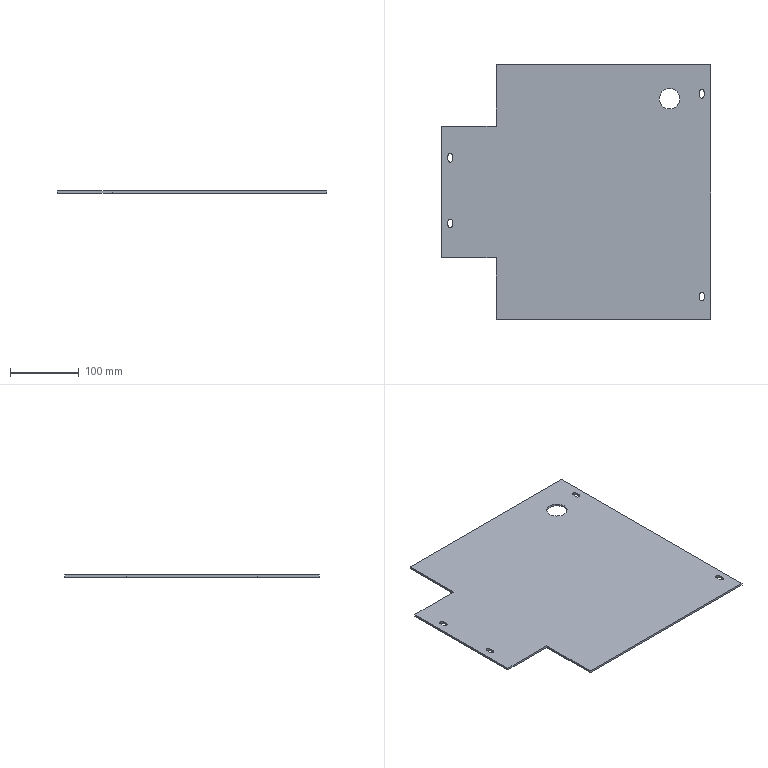Part | SolidWorks | features Cut 2, ICE 2, Extrusion 1 | 1 solid | 28 faces | box 393 x 372 x 3 mm | volume 392382 mm3 | plane 18 | cylinder 10 | commonest cylinder face diameters 6.6 x8 30 x2
STEP:
#1=CARTESIAN_POINT('',(106.5,136.,0.));
#2=VERTEX_POINT('',#1);
#3=CARTESIAN_POINT('',(136.5,136.,0.));
#4=VERTEX_POINT('',#3);
#5=CARTESIAN_POINT('',(121.5,136.,0.));
#6=DIRECTION('',(0.,0.,1.));
#7=DIRECTION('',(1.,0.,0.));
#8=AXIS2_PLACEMENT_3D('',#5,#6,#7);
#9=CIRCLE('',#8,15.);
#10=EDGE_CURVE('',#2,#4,#9,.T.);
#11=ORIENTED_EDGE('',*,*,#10,.F.);
#12=CARTESIAN_POINT('',(106.5,136.,3.));
#13=VERTEX_POINT('',#12);
#14=CARTESIAN_POINT('',(106.5,136.,-7.));
#15=DIRECTION('',(0.,0.,1.));
#16=VECTOR('',#15,1000.);
#17=LINE('',#14,#16);
#18=EDGE_CURVE('',#2,#13,#17,.T.);
#19=ORIENTED_EDGE('',*,*,#18,.T.);
#20=CARTESIAN_POINT('',(136.5,136.,3.));
#21=VERTEX_POINT('',#20);
#22=CARTESIAN_POINT('',(121.5,136.,3.));
#23=DIRECTION('',(0.,0.,1.));
#24=DIRECTION('',(1.,0.,0.));
#25=AXIS2_PLACEMENT_3D('',#22,#23,#24);
#26=CIRCLE('',#25,15.);
#27=EDGE_CURVE('',#13,#21,#26,.T.);
#28=ORIENTED_EDGE('',*,*,#27,.T.);
#29=CARTESIAN_POINT('',(136.5,136.,-7.));
#30=DIRECTION('',(0.,0.,1.));
#31=VECTOR('',#30,1000.);
#32=LINE('',#29,#31);
#33=EDGE_CURVE('',#4,#21,#32,.T.);
#34=ORIENTED_EDGE('',*,*,#33,.F.);
#35=EDGE_LOOP('',(#11,#19,#28,#34));
#36=FACE_OUTER_BOUND('',#35,.T.);
#37=CARTESIAN_POINT('',(121.5,136.,-7.));
#38=DIRECTION('',(0.,0.,1.));
#39=DIRECTION('',(1.,0.,0.));
#40=AXIS2_PLACEMENT_3D('',#37,#38,#39);
#41=CYLINDRICAL_SURFACE('',#40,15.);
#42=ADVANCED_FACE('',(#36),#41,.F.);
#43=CARTESIAN_POINT('',(-131.5,-186.,3.));
#44=VERTEX_POINT('',#43);
#45=CARTESIAN_POINT('',(181.5,-186.,3.));
#46=VERTEX_POINT('',#45);
#47=CARTESIAN_POINT('',(181.5,-186.,3.));
#48=DIRECTION('',(1.,0.,0.));
#49=VECTOR('',#48,1000.);
#50=LINE('',#47,#49);
#51=EDGE_CURVE('',#44,#46,#50,.T.);
#52=ORIENTED_EDGE('',*,*,#51,.F.);
#53=CARTESIAN_POINT('',(-131.5,-186.,0.));
#54=VERTEX_POINT('',#53);
#55=CARTESIAN_POINT('',(-131.5,-186.,-7.));
#56=DIRECTION('',(0.,0.,1.));
#57=VECTOR('',#56,1000.);
#58=LINE('',#55,#57);
#59=EDGE_CURVE('',#54,#44,#58,.T.);
#60=ORIENTED_EDGE('',*,*,#59,.F.);
#61=CARTESIAN_POINT('',(181.5,-186.,0.));
#62=VERTEX_POINT('',#61);
#63=CARTESIAN_POINT('',(181.5,-186.,0.));
#64=DIRECTION('',(1.,0.,0.));
#65=VECTOR('',#64,1000.);
#66=LINE('',#63,#65);
#67=EDGE_CURVE('',#54,#62,#66,.T.);
#68=ORIENTED_EDGE('',*,*,#67,.T.);
#69=CARTESIAN_POINT('',(181.5,-186.,3.));
#70=DIRECTION('',(0.,0.,-1.));
#71=VECTOR('',#70,1000.);
#72=LINE('',#69,#71);
#73=EDGE_CURVE('',#46,#62,#72,.T.);
#74=ORIENTED_EDGE('',*,*,#73,.F.);
#75=EDGE_LOOP('',(#52,#60,#68,#74));
#76=FACE_OUTER_BOUND('',#75,.T.);
#77=CARTESIAN_POINT('',(181.5,-186.,3.));
#78=DIRECTION('',(0.,1.,0.));
#79=DIRECTION('',(-1.,0.,0.));
#80=AXIS2_PLACEMENT_3D('',#77,#78,#79);
#81=PLANE('',#80);
#82=ADVANCED_FACE('',(#76),#81,.F.);
#83=CARTESIAN_POINT('',(181.5,186.,0.));
#84=VERTEX_POINT('',#83);
#85=CARTESIAN_POINT('',(181.5,-186.,0.));
#86=DIRECTION('',(0.,1.,0.));
#87=VECTOR('',#86,1000.);
#88=LINE('',#85,#87);
#89=EDGE_CURVE('',#62,#84,#88,.T.);
#90=ORIENTED_EDGE('',*,*,#89,.T.);
#91=CARTESIAN_POINT('',(181.5,186.,3.));
#92=VERTEX_POINT('',#91);
#93=CARTESIAN_POINT('',(181.5,186.,3.));
#94=DIRECTION('',(0.,0.,-1.));
#95=VECTOR('',#94,1000.);
#96=LINE('',#93,#95);
#97=EDGE_CURVE('',#92,#84,#96,.T.);
#98=ORIENTED_EDGE('',*,*,#97,.F.);
#99=CARTESIAN_POINT('',(181.5,-186.,3.));
#100=DIRECTION('',(0.,1.,0.));
#101=VECTOR('',#100,1000.);
#102=LINE('',#99,#101);
#103=EDGE_CURVE('',#46,#92,#102,.T.);
#104=ORIENTED_EDGE('',*,*,#103,.F.);
#105=ORIENTED_EDGE('',*,*,#73,.T.);
#106=EDGE_LOOP('',(#90,#98,#104,#105));
#107=FACE_OUTER_BOUND('',#106,.T.);
#108=CARTESIAN_POINT('',(181.5,-186.,3.));
#109=DIRECTION('',(-1.,0.,0.));
#110=DIRECTION('',(0.,0.,1.));
#111=AXIS2_PLACEMENT_3D('',#108,#109,#110);
#112=PLANE('',#111);
#113=ADVANCED_FACE('',(#107),#112,.F.);
#114=CARTESIAN_POINT('',(-131.5,186.,0.));
#115=VERTEX_POINT('',#114);
#116=CARTESIAN_POINT('',(181.5,186.,0.));
#117=DIRECTION('',(-1.,0.,0.));
#118=VECTOR('',#117,1000.);
#119=LINE('',#116,#118);
#120=EDGE_CURVE('',#84,#115,#119,.T.);
#121=ORIENTED_EDGE('',*,*,#120,.T.);
#122=CARTESIAN_POINT('',(-131.5,186.,3.));
#123=VERTEX_POINT('',#122);
#124=CARTESIAN_POINT('',(-131.5,186.,-7.));
#125=DIRECTION('',(0.,0.,1.));
#126=VECTOR('',#125,1000.);
#127=LINE('',#124,#126);
#128=EDGE_CURVE('',#115,#123,#127,.T.);
#129=ORIENTED_EDGE('',*,*,#128,.T.);
#130=CARTESIAN_POINT('',(181.5,186.,3.));
#131=DIRECTION('',(-1.,0.,0.));
#132=VECTOR('',#131,1000.);
#133=LINE('',#130,#132);
#134=EDGE_CURVE('',#92,#123,#133,.T.);
#135=ORIENTED_EDGE('',*,*,#134,.F.);
#136=ORIENTED_EDGE('',*,*,#97,.T.);
#137=EDGE_LOOP('',(#121,#129,#135,#136));
#138=FACE_OUTER_BOUND('',#137,.T.);
#139=CARTESIAN_POINT('',(181.5,186.,3.));
#140=DIRECTION('',(0.,-1.,0.));
#141=DIRECTION('',(1.,0.,0.));
#142=AXIS2_PLACEMENT_3D('',#139,#140,#141);
#143=PLANE('',#142);
#144=ADVANCED_FACE('',(#138),#143,.F.);
#145=CARTESIAN_POINT('',(165.2,-155.558,3.));
#146=VERTEX_POINT('',#145);
#147=CARTESIAN_POINT('',(171.8,-155.558,3.));
#148=VERTEX_POINT('',#147);
#149=CARTESIAN_POINT('',(168.5,-155.558,3.));
#150=DIRECTION('',(0.,0.,1.));
#151=DIRECTION('',(1.,0.,0.));
#152=AXIS2_PLACEMENT_3D('',#149,#150,#151);
#153=CIRCLE('',#152,3.3);
#154=EDGE_CURVE('',#146,#148,#153,.T.);
#155=ORIENTED_EDGE('',*,*,#154,.F.);
#156=CARTESIAN_POINT('',(165.2,-149.558,3.));
#157=VERTEX_POINT('',#156);
#158=CARTESIAN_POINT('',(165.2,-155.558,3.));
#159=DIRECTION('',(0.,-1.,0.));
#160=VECTOR('',#159,1000.);
#161=LINE('',#158,#160);
#162=EDGE_CURVE('',#157,#146,#161,.T.);
#163=ORIENTED_EDGE('',*,*,#162,.F.);
#164=CARTESIAN_POINT('',(171.8,-149.558,3.));
#165=VERTEX_POINT('',#164);
#166=CARTESIAN_POINT('',(168.5,-149.558,3.));
#167=DIRECTION('',(0.,0.,1.));
#168=DIRECTION('',(1.,0.,0.));
#169=AXIS2_PLACEMENT_3D('',#166,#167,#168);
#170=CIRCLE('',#169,3.3);
#171=EDGE_CURVE('',#165,#157,#170,.T.);
#172=ORIENTED_EDGE('',*,*,#171,.F.);
#173=CARTESIAN_POINT('',(171.8,-155.558,3.));
#174=DIRECTION('',(0.,1.,0.));
#175=VECTOR('',#174,1000.);
#176=LINE('',#173,#175);
#177=EDGE_CURVE('',#148,#165,#176,.T.);
#178=ORIENTED_EDGE('',*,*,#177,.F.);
#179=EDGE_LOOP('',(#155,#163,#172,#178));
#180=FACE_BOUND('',#179,.T.);
#181=CARTESIAN_POINT('',(165.2,140.284,3.));
#182=VERTEX_POINT('',#181);
#183=CARTESIAN_POINT('',(171.8,140.284,3.));
#184=VERTEX_POINT('',#183);
#185=CARTESIAN_POINT('',(168.5,140.284,3.));
#186=DIRECTION('',(0.,0.,1.));
#187=DIRECTION('',(1.,0.,0.));
#188=AXIS2_PLACEMENT_3D('',#185,#186,#187);
#189=CIRCLE('',#188,3.3);
#190=EDGE_CURVE('',#182,#184,#189,.T.);
#191=ORIENTED_EDGE('',*,*,#190,.F.);
#192=CARTESIAN_POINT('',(165.2,146.284,3.));
#193=VERTEX_POINT('',#192);
#194=CARTESIAN_POINT('',(165.2,140.284,3.));
#195=DIRECTION('',(0.,-1.,0.));
#196=VECTOR('',#195,1000.);
#197=LINE('',#194,#196);
#198=EDGE_CURVE('',#193,#182,#197,.T.);
#199=ORIENTED_EDGE('',*,*,#198,.F.);
#200=CARTESIAN_POINT('',(171.8,146.284,3.));
#201=VERTEX_POINT('',#200);
#202=CARTESIAN_POINT('',(168.5,146.284,3.));
#203=DIRECTION('',(0.,0.,1.));
#204=DIRECTION('',(1.,0.,0.));
#205=AXIS2_PLACEMENT_3D('',#202,#203,#204);
#206=CIRCLE('',#205,3.3);
#207=EDGE_CURVE('',#201,#193,#206,.T.);
#208=ORIENTED_EDGE('',*,*,#207,.F.);
#209=CARTESIAN_POINT('',(171.8,140.284,3.));
#210=DIRECTION('',(0.,1.,0.));
#211=VECTOR('',#210,1000.);
#212=LINE('',#209,#211);
#213=EDGE_CURVE('',#184,#201,#212,.T.);
#214=ORIENTED_EDGE('',*,*,#213,.F.);
#215=EDGE_LOOP('',(#191,#199,#208,#214));
#216=FACE_BOUND('',#215,.T.);
#217=CARTESIAN_POINT('',(-195.2,52.92,3.));
#218=VERTEX_POINT('',#217);
#219=CARTESIAN_POINT('',(-201.8,52.92,3.));
#220=VERTEX_POINT('',#219);
#221=CARTESIAN_POINT('',(-198.5,52.92,3.));
#222=DIRECTION('',(0.,0.,1.));
#223=DIRECTION('',(1.,0.,0.));
#224=AXIS2_PLACEMENT_3D('',#221,#222,#223);
#225=CIRCLE('',#224,3.3);
#226=EDGE_CURVE('',#218,#220,#225,.T.);
#227=ORIENTED_EDGE('',*,*,#226,.F.);
#228=CARTESIAN_POINT('',(-195.2,46.92,3.));
#229=VERTEX_POINT('',#228);
#230=CARTESIAN_POINT('',(-195.2,52.92,3.));
#231=DIRECTION('',(0.,1.,0.));
#232=VECTOR('',#231,1000.);
#233=LINE('',#230,#232);
#234=EDGE_CURVE('',#229,#218,#233,.T.);
#235=ORIENTED_EDGE('',*,*,#234,.F.);
#236=CARTESIAN_POINT('',(-201.8,46.92,3.));
#237=VERTEX_POINT('',#236);
#238=CARTESIAN_POINT('',(-198.5,46.92,3.));
#239=DIRECTION('',(0.,0.,1.));
#240=DIRECTION('',(1.,0.,0.));
#241=AXIS2_PLACEMENT_3D('',#238,#239,#240);
#242=CIRCLE('',#241,3.3);
#243=EDGE_CURVE('',#237,#229,#242,.T.);
#244=ORIENTED_EDGE('',*,*,#243,.F.);
#245=CARTESIAN_POINT('',(-201.8,52.92,3.));
#246=DIRECTION('',(0.,-1.,0.));
#247=VECTOR('',#246,1000.);
#248=LINE('',#245,#247);
#249=EDGE_CURVE('',#220,#237,#248,.T.);
#250=ORIENTED_EDGE('',*,*,#249,.F.);
#251=EDGE_LOOP('',(#227,#235,#244,#250));
#252=FACE_BOUND('',#251,.T.);
#253=CARTESIAN_POINT('',(-201.8,-48.715,3.));
#254=VERTEX_POINT('',#253);
#255=CARTESIAN_POINT('',(-195.2,-48.715,3.));
#256=VERTEX_POINT('',#255);
#257=CARTESIAN_POINT('',(-198.5,-48.715,3.));
#258=DIRECTION('',(0.,0.,1.));
#259=DIRECTION('',(1.,0.,0.));
#260=AXIS2_PLACEMENT_3D('',#257,#258,#259);
#261=CIRCLE('',#260,3.3);
#262=EDGE_CURVE('',#254,#256,#261,.T.);
#263=ORIENTED_EDGE('',*,*,#262,.F.);
#264=CARTESIAN_POINT('',(-201.8,-42.715,3.));
#265=VERTEX_POINT('',#264);
#266=CARTESIAN_POINT('',(-201.8,-48.715,3.));
#267=DIRECTION('',(0.,-1.,0.));
#268=VECTOR('',#267,1000.);
#269=LINE('',#266,#268);
#270=EDGE_CURVE('',#265,#254,#269,.T.);
#271=ORIENTED_EDGE('',*,*,#270,.F.);
#272=CARTESIAN_POINT('',(-195.2,-42.715,3.));
#273=VERTEX_POINT('',#272);
#274=CARTESIAN_POINT('',(-198.5,-42.715,3.));
#275=DIRECTION('',(0.,0.,1.));
#276=DIRECTION('',(1.,0.,0.));
#277=AXIS2_PLACEMENT_3D('',#274,#275,#276);
#278=CIRCLE('',#277,3.3);
#279=EDGE_CURVE('',#273,#265,#278,.T.);
#280=ORIENTED_EDGE('',*,*,#279,.F.);
#281=CARTESIAN_POINT('',(-195.2,-48.715,3.));
#282=DIRECTION('',(0.,1.,0.));
#283=VECTOR('',#282,1000.);
#284=LINE('',#281,#283);
#285=EDGE_CURVE('',#256,#273,#284,.T.);
#286=ORIENTED_EDGE('',*,*,#285,.F.);
#287=EDGE_LOOP('',(#263,#271,#280,#286));
#288=FACE_BOUND('',#287,.T.);
#289=CARTESIAN_POINT('',(-131.5,-96.,3.));
#290=VERTEX_POINT('',#289);
#291=CARTESIAN_POINT('',(-211.5,-96.,3.));
#292=VERTEX_POINT('',#291);
#293=CARTESIAN_POINT('',(-131.5,-96.,3.));
#294=DIRECTION('',(-1.,0.,0.));
#295=VECTOR('',#294,1000.);
#296=LINE('',#293,#295);
#297=EDGE_CURVE('',#290,#292,#296,.T.);
#298=ORIENTED_EDGE('',*,*,#297,.F.);
#299=CARTESIAN_POINT('',(-131.5,-96.,3.));
#300=DIRECTION('',(0.,1.,0.));
#301=VECTOR('',#300,1000.);
#302=LINE('',#299,#301);
#303=EDGE_CURVE('',#44,#290,#302,.T.);
#304=ORIENTED_EDGE('',*,*,#303,.F.);
#305=ORIENTED_EDGE('',*,*,#51,.T.);
#306=ORIENTED_EDGE('',*,*,#103,.T.);
#307=ORIENTED_EDGE('',*,*,#134,.T.);
#308=CARTESIAN_POINT('',(-131.5,96.,3.));
#309=VERTEX_POINT('',#308);
#310=CARTESIAN_POINT('',(-131.5,96.,3.));
#311=DIRECTION('',(0.,1.,0.));
#312=VECTOR('',#311,1000.);
#313=LINE('',#310,#312);
#314=EDGE_CURVE('',#309,#123,#313,.T.);
#315=ORIENTED_EDGE('',*,*,#314,.F.);
#316=CARTESIAN_POINT('',(-211.5,96.,3.));
#317=VERTEX_POINT('',#316);
#318=CARTESIAN_POINT('',(-131.5,96.,3.));
#319=DIRECTION('',(1.,0.,0.));
#320=VECTOR('',#319,1000.);
#321=LINE('',#318,#320);
#322=EDGE_CURVE('',#317,#309,#321,.T.);
#323=ORIENTED_EDGE('',*,*,#322,.F.);
#324=CARTESIAN_POINT('',(-211.5,-96.,3.));
#325=DIRECTION('',(0.,1.,0.));
#326=VECTOR('',#325,1000.);
#327=LINE('',#324,#326);
#328=EDGE_CURVE('',#292,#317,#327,.T.);
#329=ORIENTED_EDGE('',*,*,#328,.F.);
#330=EDGE_LOOP('',(#298,#304,#305,#306,#307,#315,#323,#329));
#331=FACE_OUTER_BOUND('',#330,.T.);
#332=CARTESIAN_POINT('',(121.5,136.,3.));
#333=DIRECTION('',(0.,0.,1.));
#334=DIRECTION('',(1.,0.,0.));
#335=AXIS2_PLACEMENT_3D('',#332,#333,#334);
#336=CIRCLE('',#335,15.);
#337=EDGE_CURVE('',#21,#13,#336,.T.);
#338=ORIENTED_EDGE('',*,*,#337,.F.);
#339=ORIENTED_EDGE('',*,*,#27,.F.);
#340=EDGE_LOOP('',(#338,#339));
#341=FACE_BOUND('',#340,.T.);
#342=CARTESIAN_POINT('',(0.,0.,3.));
#343=DIRECTION('',(0.,0.,1.));
#344=DIRECTION('',(1.,0.,0.));
#345=AXIS2_PLACEMENT_3D('',#342,#343,#344);
#346=PLANE('',#345);
#347=ADVANCED_FACE('',(#180,#216,#252,#288,#331,#341),#346,.T.);
#348=CARTESIAN_POINT('',(165.2,-149.558,0.));
#349=VERTEX_POINT('',#348);
#350=CARTESIAN_POINT('',(165.2,-155.558,0.));
#351=VERTEX_POINT('',#350);
#352=CARTESIAN_POINT('',(165.2,0.,0.));
#353=DIRECTION('',(0.,-1.,0.));
#354=VECTOR('',#353,1000.);
#355=LINE('',#352,#354);
#356=EDGE_CURVE('',#349,#351,#355,.T.);
#357=ORIENTED_EDGE('',*,*,#356,.T.);
#358=CARTESIAN_POINT('',(171.8,-155.558,0.));
#359=VERTEX_POINT('',#358);
#360=CARTESIAN_POINT('',(168.5,-155.558,0.));
#361=DIRECTION('',(0.,0.,1.));
#362=DIRECTION('',(1.,0.,0.));
#363=AXIS2_PLACEMENT_3D('',#360,#361,#362);
#364=CIRCLE('',#363,3.3);
#365=EDGE_CURVE('',#351,#359,#364,.T.);
#366=ORIENTED_EDGE('',*,*,#365,.T.);
#367=CARTESIAN_POINT('',(171.8,-149.558,0.));
#368=VERTEX_POINT('',#367);
#369=CARTESIAN_POINT('',(171.8,0.,0.));
#370=DIRECTION('',(0.,1.,0.));
#371=VECTOR('',#370,1000.);
#372=LINE('',#369,#371);
#373=EDGE_CURVE('',#359,#368,#372,.T.);
#374=ORIENTED_EDGE('',*,*,#373,.T.);
#375=CARTESIAN_POINT('',(168.5,-149.558,0.));
#376=DIRECTION('',(0.,0.,1.));
#377=DIRECTION('',(1.,0.,0.));
#378=AXIS2_PLACEMENT_3D('',#375,#376,#377);
#379=CIRCLE('',#378,3.3);
#380=EDGE_CURVE('',#368,#349,#379,.T.);
#381=ORIENTED_EDGE('',*,*,#380,.T.);
#382=EDGE_LOOP('',(#357,#366,#374,#381));
#383=FACE_BOUND('',#382,.T.);
#384=CARTESIAN_POINT('',(165.2,146.284,0.));
#385=VERTEX_POINT('',#384);
#386=CARTESIAN_POINT('',(165.2,140.284,0.));
#387=VERTEX_POINT('',#386);
#388=CARTESIAN_POINT('',(165.2,0.,0.));
#389=DIRECTION('',(0.,-1.,0.));
#390=VECTOR('',#389,1000.);
#391=LINE('',#388,#390);
#392=EDGE_CURVE('',#385,#387,#391,.T.);
#393=ORIENTED_EDGE('',*,*,#392,.T.);
#394=CARTESIAN_POINT('',(171.8,140.284,0.));
#395=VERTEX_POINT('',#394);
#396=CARTESIAN_POINT('',(168.5,140.284,0.));
#397=DIRECTION('',(0.,0.,1.));
#398=DIRECTION('',(1.,0.,0.));
#399=AXIS2_PLACEMENT_3D('',#396,#397,#398);
#400=CIRCLE('',#399,3.3);
#401=EDGE_CURVE('',#387,#395,#400,.T.);
#402=ORIENTED_EDGE('',*,*,#401,.T.);
#403=CARTESIAN_POINT('',(171.8,146.284,0.));
#404=VERTEX_POINT('',#403);
#405=CARTESIAN_POINT('',(171.8,0.,0.));
#406=DIRECTION('',(0.,1.,0.));
#407=VECTOR('',#406,1000.);
#408=LINE('',#405,#407);
#409=EDGE_CURVE('',#395,#404,#408,.T.);
#410=ORIENTED_EDGE('',*,*,#409,.T.);
#411=CARTESIAN_POINT('',(168.5,146.284,0.));
#412=DIRECTION('',(0.,0.,1.));
#413=DIRECTION('',(1.,0.,0.));
#414=AXIS2_PLACEMENT_3D('',#411,#412,#413);
#415=CIRCLE('',#414,3.3);
#416=EDGE_CURVE('',#404,#385,#415,.T.);
#417=ORIENTED_EDGE('',*,*,#416,.T.);
#418=EDGE_LOOP('',(#393,#402,#410,#417));
#419=FACE_BOUND('',#418,.T.);
#420=CARTESIAN_POINT('',(-195.2,46.92,0.));
#421=VERTEX_POINT('',#420);
#422=CARTESIAN_POINT('',(-195.2,52.92,0.));
#423=VERTEX_POINT('',#422);
#424=CARTESIAN_POINT('',(-195.2,0.,0.));
#425=DIRECTION('',(0.,1.,0.));
#426=VECTOR('',#425,1000.);
#427=LINE('',#424,#426);
#428=EDGE_CURVE('',#421,#423,#427,.T.);
#429=ORIENTED_EDGE('',*,*,#428,.T.);
#430=CARTESIAN_POINT('',(-201.8,52.92,0.));
#431=VERTEX_POINT('',#430);
#432=CARTESIAN_POINT('',(-198.5,52.92,0.));
#433=DIRECTION('',(0.,0.,1.));
#434=DIRECTION('',(1.,0.,0.));
#435=AXIS2_PLACEMENT_3D('',#432,#433,#434);
#436=CIRCLE('',#435,3.3);
#437=EDGE_CURVE('',#423,#431,#436,.T.);
#438=ORIENTED_EDGE('',*,*,#437,.T.);
#439=CARTESIAN_POINT('',(-201.8,46.92,0.));
#440=VERTEX_POINT('',#439);
#441=CARTESIAN_POINT('',(-201.8,0.,0.));
#442=DIRECTION('',(0.,-1.,0.));
#443=VECTOR('',#442,1000.);
#444=LINE('',#441,#443);
#445=EDGE_CURVE('',#431,#440,#444,.T.);
#446=ORIENTED_EDGE('',*,*,#445,.T.);
#447=CARTESIAN_POINT('',(-198.5,46.92,0.));
#448=DIRECTION('',(0.,0.,1.));
#449=DIRECTION('',(1.,0.,0.));
#450=AXIS2_PLACEMENT_3D('',#447,#448,#449);
#451=CIRCLE('',#450,3.3);
#452=EDGE_CURVE('',#440,#421,#451,.T.);
#453=ORIENTED_EDGE('',*,*,#452,.T.);
#454=EDGE_LOOP('',(#429,#438,#446,#453));
#455=FACE_BOUND('',#454,.T.);
#456=CARTESIAN_POINT('',(-201.8,-42.715,0.));
#457=VERTEX_POINT('',#456);
#458=CARTESIAN_POINT('',(-201.8,-48.715,0.));
#459=VERTEX_POINT('',#458);
#460=CARTESIAN_POINT('',(-201.8,0.,0.));
#461=DIRECTION('',(0.,-1.,0.));
#462=VECTOR('',#461,1000.);
#463=LINE('',#460,#462);
#464=EDGE_CURVE('',#457,#459,#463,.T.);
#465=ORIENTED_EDGE('',*,*,#464,.T.);
#466=CARTESIAN_POINT('',(-195.2,-48.715,0.));
#467=VERTEX_POINT('',#466);
#468=CARTESIAN_POINT('',(-198.5,-48.715,0.));
#469=DIRECTION('',(0.,0.,1.));
#470=DIRECTION('',(1.,0.,0.));
#471=AXIS2_PLACEMENT_3D('',#468,#469,#470);
#472=CIRCLE('',#471,3.3);
#473=EDGE_CURVE('',#459,#467,#472,.T.);
#474=ORIENTED_EDGE('',*,*,#473,.T.);
#475=CARTESIAN_POINT('',(-195.2,-42.715,0.));
#476=VERTEX_POINT('',#475);
#477=CARTESIAN_POINT('',(-195.2,0.,0.));
#478=DIRECTION('',(0.,1.,0.));
#479=VECTOR('',#478,1000.);
#480=LINE('',#477,#479);
#481=EDGE_CURVE('',#467,#476,#480,.T.);
#482=ORIENTED_EDGE('',*,*,#481,.T.);
#483=CARTESIAN_POINT('',(-198.5,-42.715,0.));
#484=DIRECTION('',(0.,0.,1.));
#485=DIRECTION('',(1.,0.,0.));
#486=AXIS2_PLACEMENT_3D('',#483,#484,#485);
#487=CIRCLE('',#486,3.3);
#488=EDGE_CURVE('',#476,#457,#487,.T.);
#489=ORIENTED_EDGE('',*,*,#488,.T.);
#490=EDGE_LOOP('',(#465,#474,#482,#489));
#491=FACE_BOUND('',#490,.T.);
#492=CARTESIAN_POINT('',(121.5,136.,0.));
#493=DIRECTION('',(0.,0.,1.));
#494=DIRECTION('',(1.,0.,0.));
#495=AXIS2_PLACEMENT_3D('',#492,#493,#494);
#496=CIRCLE('',#495,15.);
#497=EDGE_CURVE('',#4,#2,#496,.T.);
#498=ORIENTED_EDGE('',*,*,#497,.T.);
#499=ORIENTED_EDGE('',*,*,#10,.T.);
#500=EDGE_LOOP('',(#498,#499));
#501=FACE_BOUND('',#500,.T.);
#502=CARTESIAN_POINT('',(-131.5,-96.,0.));
#503=VERTEX_POINT('',#502);
#504=CARTESIAN_POINT('',(-131.5,0.,0.));
#505=DIRECTION('',(0.,1.,0.));
#506=VECTOR('',#505,1000.);
#507=LINE('',#504,#506);
#508=EDGE_CURVE('',#54,#503,#507,.T.);
#509=ORIENTED_EDGE('',*,*,#508,.T.);
#510=CARTESIAN_POINT('',(-211.5,-96.,0.));
#511=VERTEX_POINT('',#510);
#512=CARTESIAN_POINT('',(0.,-96.,0.));
#513=DIRECTION('',(-1.,0.,0.));
#514=VECTOR('',#513,1000.);
#515=LINE('',#512,#514);
#516=EDGE_CURVE('',#503,#511,#515,.T.);
#517=ORIENTED_EDGE('',*,*,#516,.T.);
#518=CARTESIAN_POINT('',(-211.5,96.,0.));
#519=VERTEX_POINT('',#518);
#520=CARTESIAN_POINT('',(-211.5,96.,0.));
#521=DIRECTION('',(0.,-1.,0.));
#522=VECTOR('',#521,1000.);
#523=LINE('',#520,#522);
#524=EDGE_CURVE('',#519,#511,#523,.T.);
#525=ORIENTED_EDGE('',*,*,#524,.F.);
#526=CARTESIAN_POINT('',(-131.5,96.,0.));
#527=VERTEX_POINT('',#526);
#528=CARTESIAN_POINT('',(0.,96.,0.));
#529=DIRECTION('',(1.,0.,0.));
#530=VECTOR('',#529,1000.);
#531=LINE('',#528,#530);
#532=EDGE_CURVE('',#519,#527,#531,.T.);
#533=ORIENTED_EDGE('',*,*,#532,.T.);
#534=CARTESIAN_POINT('',(-131.5,0.,0.));
#535=DIRECTION('',(0.,1.,0.));
#536=VECTOR('',#535,1000.);
#537=LINE('',#534,#536);
#538=EDGE_CURVE('',#527,#115,#537,.T.);
#539=ORIENTED_EDGE('',*,*,#538,.T.);
#540=ORIENTED_EDGE('',*,*,#120,.F.);
#541=ORIENTED_EDGE('',*,*,#89,.F.);
#542=ORIENTED_EDGE('',*,*,#67,.F.);
#543=EDGE_LOOP('',(#509,#517,#525,#533,#539,#540,#541,#542));
#544=FACE_OUTER_BOUND('',#543,.T.);
#545=CARTESIAN_POINT('',(0.,0.,0.));
#546=DIRECTION('',(0.,0.,1.));
#547=DIRECTION('',(1.,0.,0.));
#548=AXIS2_PLACEMENT_3D('',#545,#546,#547);
#549=PLANE('',#548);
#550=ADVANCED_FACE('',(#383,#419,#455,#491,#501,#544),#549,.F.);
#551=ORIENTED_EDGE('',*,*,#18,.F.);
#552=ORIENTED_EDGE('',*,*,#497,.F.);
#553=ORIENTED_EDGE('',*,*,#33,.T.);
#554=ORIENTED_EDGE('',*,*,#337,.T.);
#555=EDGE_LOOP('',(#551,#552,#553,#554));
#556=FACE_OUTER_BOUND('',#555,.T.);
#557=CARTESIAN_POINT('',(121.5,136.,-7.));
#558=DIRECTION('',(0.,0.,1.));
#559=DIRECTION('',(1.,0.,0.));
#560=AXIS2_PLACEMENT_3D('',#557,#558,#559);
#561=CYLINDRICAL_SURFACE('',#560,15.);
#562=ADVANCED_FACE('',(#556),#561,.F.);
#563=CARTESIAN_POINT('',(-131.5,96.,-7.));
#564=DIRECTION('',(0.,0.,1.));
#565=VECTOR('',#564,1000.);
#566=LINE('',#563,#565);
#567=EDGE_CURVE('',#527,#309,#566,.T.);
#568=ORIENTED_EDGE('',*,*,#567,.T.);
#569=ORIENTED_EDGE('',*,*,#314,.T.);
#570=ORIENTED_EDGE('',*,*,#128,.F.);
#571=ORIENTED_EDGE('',*,*,#538,.F.);
#572=EDGE_LOOP('',(#568,#569,#570,#571));
#573=FACE_OUTER_BOUND('',#572,.T.);
#574=CARTESIAN_POINT('',(-131.5,96.,-7.));
#575=DIRECTION('',(1.,0.,0.));
#576=DIRECTION('',(0.,0.,-1.));
#577=AXIS2_PLACEMENT_3D('',#574,#575,#576);
#578=PLANE('',#577);
#579=ADVANCED_FACE('',(#573),#578,.F.);
#580=ORIENTED_EDGE('',*,*,#532,.F.);
#581=CARTESIAN_POINT('',(-211.5,96.,3.));
#582=DIRECTION('',(0.,0.,-1.));
#583=VECTOR('',#582,1000.);
#584=LINE('',#581,#583);
#585=EDGE_CURVE('',#317,#519,#584,.T.);
#586=ORIENTED_EDGE('',*,*,#585,.F.);
#587=ORIENTED_EDGE('',*,*,#322,.T.);
#588=ORIENTED_EDGE('',*,*,#567,.F.);
#589=EDGE_LOOP('',(#580,#586,#587,#588));
#590=FACE_OUTER_BOUND('',#589,.T.);
#591=CARTESIAN_POINT('',(-131.5,96.,-7.));
#592=DIRECTION('',(0.,-1.,0.));
#593=DIRECTION('',(0.,0.,-1.));
#594=AXIS2_PLACEMENT_3D('',#591,#592,#593);
#595=PLANE('',#594);
#596=ADVANCED_FACE('',(#590),#595,.F.);
#597=CARTESIAN_POINT('',(-131.5,-96.,-7.));
#598=DIRECTION('',(0.,0.,1.));
#599=VECTOR('',#598,1000.);
#600=LINE('',#597,#599);
#601=EDGE_CURVE('',#503,#290,#600,.T.);
#602=ORIENTED_EDGE('',*,*,#601,.T.);
#603=ORIENTED_EDGE('',*,*,#297,.T.);
#604=CARTESIAN_POINT('',(-211.5,-96.,0.));
#605=DIRECTION('',(0.,0.,1.));
#606=VECTOR('',#605,1000.);
#607=LINE('',#604,#606);
#608=EDGE_CURVE('',#511,#292,#607,.T.);
#609=ORIENTED_EDGE('',*,*,#608,.F.);
#610=ORIENTED_EDGE('',*,*,#516,.F.);
#611=EDGE_LOOP('',(#602,#603,#609,#610));
#612=FACE_OUTER_BOUND('',#611,.T.);
#613=CARTESIAN_POINT('',(-131.5,-96.,-7.));
#614=DIRECTION('',(0.,1.,0.));
#615=DIRECTION('',(-1.,0.,0.));
#616=AXIS2_PLACEMENT_3D('',#613,#614,#615);
#617=PLANE('',#616);
#618=ADVANCED_FACE('',(#612),#617,.F.);
#619=ORIENTED_EDGE('',*,*,#59,.T.);
#620=ORIENTED_EDGE('',*,*,#303,.T.);
#621=ORIENTED_EDGE('',*,*,#601,.F.);
#622=ORIENTED_EDGE('',*,*,#508,.F.);
#623=EDGE_LOOP('',(#619,#620,#621,#622));
#624=FACE_OUTER_BOUND('',#623,.T.);
#625=CARTESIAN_POINT('',(-131.5,-96.,-7.));
#626=DIRECTION('',(1.,0.,0.));
#627=DIRECTION('',(0.,0.,-1.));
#628=AXIS2_PLACEMENT_3D('',#625,#626,#627);
#629=PLANE('',#628);
#630=ADVANCED_FACE('',(#624),#629,.F.);
#631=ORIENTED_EDGE('',*,*,#585,.T.);
#632=ORIENTED_EDGE('',*,*,#524,.T.);
#633=ORIENTED_EDGE('',*,*,#608,.T.);
#634=ORIENTED_EDGE('',*,*,#328,.T.);
#635=EDGE_LOOP('',(#631,#632,#633,#634));
#636=FACE_OUTER_BOUND('',#635,.T.);
#637=CARTESIAN_POINT('',(-211.5,0.,0.));
#638=DIRECTION('',(-1.,0.,0.));
#639=DIRECTION('',(0.,0.,1.));
#640=AXIS2_PLACEMENT_3D('',#637,#638,#639);
#641=PLANE('',#640);
#642=ADVANCED_FACE('',(#636),#641,.T.);
#643=CARTESIAN_POINT('',(-201.8,-48.715,-7.));
#644=DIRECTION('',(0.,0.,1.));
#645=VECTOR('',#644,1000.);
#646=LINE('',#643,#645);
#647=EDGE_CURVE('',#459,#254,#646,.T.);
#648=ORIENTED_EDGE('',*,*,#647,.T.);
#649=ORIENTED_EDGE('',*,*,#262,.T.);
#650=CARTESIAN_POINT('',(-195.2,-48.715,-7.));
#651=DIRECTION('',(0.,0.,1.));
#652=VECTOR('',#651,1000.);
#653=LINE('',#650,#652);
#654=EDGE_CURVE('',#467,#256,#653,.T.);
#655=ORIENTED_EDGE('',*,*,#654,.F.);
#656=ORIENTED_EDGE('',*,*,#473,.F.);
#657=EDGE_LOOP('',(#648,#649,#655,#656));
#658=FACE_OUTER_BOUND('',#657,.T.);
#659=CARTESIAN_POINT('',(-198.5,-48.715,-7.));
#660=DIRECTION('',(0.,0.,1.));
#661=DIRECTION('',(1.,0.,0.));
#662=AXIS2_PLACEMENT_3D('',#659,#660,#661);
#663=CYLINDRICAL_SURFACE('',#662,3.3);
#664=ADVANCED_FACE('',(#658),#663,.F.);
#665=CARTESIAN_POINT('',(-201.8,-42.715,-7.));
#666=DIRECTION('',(0.,0.,1.));
#667=VECTOR('',#666,1000.);
#668=LINE('',#665,#667);
#669=EDGE_CURVE('',#457,#265,#668,.T.);
#670=ORIENTED_EDGE('',*,*,#669,.T.);
#671=ORIENTED_EDGE('',*,*,#270,.T.);
#672=ORIENTED_EDGE('',*,*,#647,.F.);
#673=ORIENTED_EDGE('',*,*,#464,.F.);
#674=EDGE_LOOP('',(#670,#671,#672,#673));
#675=FACE_OUTER_BOUND('',#674,.T.);
#676=CARTESIAN_POINT('',(-201.8,-48.715,-7.));
#677=DIRECTION('',(-1.,0.,0.));
#678=DIRECTION('',(0.,-1.,0.));
#679=AXIS2_PLACEMENT_3D('',#676,#677,#678);
#680=PLANE('',#679);
#681=ADVANCED_FACE('',(#675),#680,.F.);
#682=CARTESIAN_POINT('',(-195.2,-42.715,-7.));
#683=DIRECTION('',(0.,0.,1.));
#684=VECTOR('',#683,1000.);
#685=LINE('',#682,#684);
#686=EDGE_CURVE('',#476,#273,#685,.T.);
#687=ORIENTED_EDGE('',*,*,#686,.T.);
#688=ORIENTED_EDGE('',*,*,#279,.T.);
#689=ORIENTED_EDGE('',*,*,#669,.F.);
#690=ORIENTED_EDGE('',*,*,#488,.F.);
#691=EDGE_LOOP('',(#687,#688,#689,#690));
#692=FACE_OUTER_BOUND('',#691,.T.);
#693=CARTESIAN_POINT('',(-198.5,-42.715,-7.));
#694=DIRECTION('',(0.,0.,1.));
#695=DIRECTION('',(1.,0.,0.));
#696=AXIS2_PLACEMENT_3D('',#693,#694,#695);
#697=CYLINDRICAL_SURFACE('',#696,3.3);
#698=ADVANCED_FACE('',(#692),#697,.F.);
#699=ORIENTED_EDGE('',*,*,#654,.T.);
#700=ORIENTED_EDGE('',*,*,#285,.T.);
#701=ORIENTED_EDGE('',*,*,#686,.F.);
#702=ORIENTED_EDGE('',*,*,#481,.F.);
#703=EDGE_LOOP('',(#699,#700,#701,#702));
#704=FACE_OUTER_BOUND('',#703,.T.);
#705=CARTESIAN_POINT('',(-195.2,-48.715,-7.));
#706=DIRECTION('',(1.,0.,0.));
#707=DIRECTION('',(0.,1.,0.));
#708=AXIS2_PLACEMENT_3D('',#705,#706,#707);
#709=PLANE('',#708);
#710=ADVANCED_FACE('',(#704),#709,.F.);
#711=CARTESIAN_POINT('',(-195.2,52.92,-7.));
#712=DIRECTION('',(0.,0.,1.));
#713=VECTOR('',#712,1000.);
#714=LINE('',#711,#713);
#715=EDGE_CURVE('',#423,#218,#714,.T.);
#716=ORIENTED_EDGE('',*,*,#715,.T.);
#717=ORIENTED_EDGE('',*,*,#226,.T.);
#718=CARTESIAN_POINT('',(-201.8,52.92,-7.));
#719=DIRECTION('',(0.,0.,1.));
#720=VECTOR('',#719,1000.);
#721=LINE('',#718,#720);
#722=EDGE_CURVE('',#431,#220,#721,.T.);
#723=ORIENTED_EDGE('',*,*,#722,.F.);
#724=ORIENTED_EDGE('',*,*,#437,.F.);
#725=EDGE_LOOP('',(#716,#717,#723,#724));
#726=FACE_OUTER_BOUND('',#725,.T.);
#727=CARTESIAN_POINT('',(-198.5,52.92,-7.));
#728=DIRECTION('',(0.,0.,1.));
#729=DIRECTION('',(1.,0.,0.));
#730=AXIS2_PLACEMENT_3D('',#727,#728,#729);
#731=CYLINDRICAL_SURFACE('',#730,3.3);
#732=ADVANCED_FACE('',(#726),#731,.F.);
#733=CARTESIAN_POINT('',(-195.2,46.92,-7.));
#734=DIRECTION('',(0.,0.,1.));
#735=VECTOR('',#734,1000.);
#736=LINE('',#733,#735);
#737=EDGE_CURVE('',#421,#229,#736,.T.);
#738=ORIENTED_EDGE('',*,*,#737,.T.);
#739=ORIENTED_EDGE('',*,*,#234,.T.);
#740=ORIENTED_EDGE('',*,*,#715,.F.);
#741=ORIENTED_EDGE('',*,*,#428,.F.);
#742=EDGE_LOOP('',(#738,#739,#740,#741));
#743=FACE_OUTER_BOUND('',#742,.T.);
#744=CARTESIAN_POINT('',(-195.2,52.92,-7.));
#745=DIRECTION('',(1.,0.,0.));
#746=DIRECTION('',(0.,0.,-1.));
#747=AXIS2_PLACEMENT_3D('',#744,#745,#746);
#748=PLANE('',#747);
#749=ADVANCED_FACE('',(#743),#748,.F.);
#750=CARTESIAN_POINT('',(-201.8,46.92,-7.));
#751=DIRECTION('',(0.,0.,1.));
#752=VECTOR('',#751,1000.);
#753=LINE('',#750,#752);
#754=EDGE_CURVE('',#440,#237,#753,.T.);
#755=ORIENTED_EDGE('',*,*,#754,.T.);
#756=ORIENTED_EDGE('',*,*,#243,.T.);
#757=ORIENTED_EDGE('',*,*,#737,.F.);
#758=ORIENTED_EDGE('',*,*,#452,.F.);
#759=EDGE_LOOP('',(#755,#756,#757,#758));
#760=FACE_OUTER_BOUND('',#759,.T.);
#761=CARTESIAN_POINT('',(-198.5,46.92,-7.));
#762=DIRECTION('',(0.,0.,1.));
#763=DIRECTION('',(1.,0.,0.));
#764=AXIS2_PLACEMENT_3D('',#761,#762,#763);
#765=CYLINDRICAL_SURFACE('',#764,3.3);
#766=ADVANCED_FACE('',(#760),#765,.F.);
#767=ORIENTED_EDGE('',*,*,#722,.T.);
#768=ORIENTED_EDGE('',*,*,#249,.T.);
#769=ORIENTED_EDGE('',*,*,#754,.F.);
#770=ORIENTED_EDGE('',*,*,#445,.F.);
#771=EDGE_LOOP('',(#767,#768,#769,#770));
#772=FACE_OUTER_BOUND('',#771,.T.);
#773=CARTESIAN_POINT('',(-201.8,52.92,-7.));
#774=DIRECTION('',(-1.,0.,0.));
#775=DIRECTION('',(0.,0.,1.));
#776=AXIS2_PLACEMENT_3D('',#773,#774,#775);
#777=PLANE('',#776);
#778=ADVANCED_FACE('',(#772),#777,.F.);
#779=CARTESIAN_POINT('',(165.2,140.284,-7.));
#780=DIRECTION('',(0.,0.,1.));
#781=VECTOR('',#780,1000.);
#782=LINE('',#779,#781);
#783=EDGE_CURVE('',#387,#182,#782,.T.);
#784=ORIENTED_EDGE('',*,*,#783,.T.);
#785=ORIENTED_EDGE('',*,*,#190,.T.);
#786=CARTESIAN_POINT('',(171.8,140.284,-7.));
#787=DIRECTION('',(0.,0.,1.));
#788=VECTOR('',#787,1000.);
#789=LINE('',#786,#788);
#790=EDGE_CURVE('',#395,#184,#789,.T.);
#791=ORIENTED_EDGE('',*,*,#790,.F.);
#792=ORIENTED_EDGE('',*,*,#401,.F.);
#793=EDGE_LOOP('',(#784,#785,#791,#792));
#794=FACE_OUTER_BOUND('',#793,.T.);
#795=CARTESIAN_POINT('',(168.5,140.284,-7.));
#796=DIRECTION('',(0.,0.,1.));
#797=DIRECTION('',(1.,0.,0.));
#798=AXIS2_PLACEMENT_3D('',#795,#796,#797);
#799=CYLINDRICAL_SURFACE('',#798,3.3);
#800=ADVANCED_FACE('',(#794),#799,.F.);
#801=CARTESIAN_POINT('',(165.2,146.284,-7.));
#802=DIRECTION('',(0.,0.,1.));
#803=VECTOR('',#802,1000.);
#804=LINE('',#801,#803);
#805=EDGE_CURVE('',#385,#193,#804,.T.);
#806=ORIENTED_EDGE('',*,*,#805,.T.);
#807=ORIENTED_EDGE('',*,*,#198,.T.);
#808=ORIENTED_EDGE('',*,*,#783,.F.);
#809=ORIENTED_EDGE('',*,*,#392,.F.);
#810=EDGE_LOOP('',(#806,#807,#808,#809));
#811=FACE_OUTER_BOUND('',#810,.T.);
#812=CARTESIAN_POINT('',(165.2,140.284,-7.));
#813=DIRECTION('',(-1.,0.,0.));
#814=DIRECTION('',(0.,0.,1.));
#815=AXIS2_PLACEMENT_3D('',#812,#813,#814);
#816=PLANE('',#815);
#817=ADVANCED_FACE('',(#811),#816,.F.);
#818=CARTESIAN_POINT('',(171.8,146.284,-7.));
#819=DIRECTION('',(0.,0.,1.));
#820=VECTOR('',#819,1000.);
#821=LINE('',#818,#820);
#822=EDGE_CURVE('',#404,#201,#821,.T.);
#823=ORIENTED_EDGE('',*,*,#822,.T.);
#824=ORIENTED_EDGE('',*,*,#207,.T.);
#825=ORIENTED_EDGE('',*,*,#805,.F.);
#826=ORIENTED_EDGE('',*,*,#416,.F.);
#827=EDGE_LOOP('',(#823,#824,#825,#826));
#828=FACE_OUTER_BOUND('',#827,.T.);
#829=CARTESIAN_POINT('',(168.5,146.284,-7.));
#830=DIRECTION('',(0.,0.,1.));
#831=DIRECTION('',(1.,0.,0.));
#832=AXIS2_PLACEMENT_3D('',#829,#830,#831);
#833=CYLINDRICAL_SURFACE('',#832,3.3);
#834=ADVANCED_FACE('',(#828),#833,.F.);
#835=ORIENTED_EDGE('',*,*,#790,.T.);
#836=ORIENTED_EDGE('',*,*,#213,.T.);
#837=ORIENTED_EDGE('',*,*,#822,.F.);
#838=ORIENTED_EDGE('',*,*,#409,.F.);
#839=EDGE_LOOP('',(#835,#836,#837,#838));
#840=FACE_OUTER_BOUND('',#839,.T.);
#841=CARTESIAN_POINT('',(171.8,140.284,-7.));
#842=DIRECTION('',(1.,0.,0.));
#843=DIRECTION('',(0.,0.,-1.));
#844=AXIS2_PLACEMENT_3D('',#841,#842,#843);
#845=PLANE('',#844);
#846=ADVANCED_FACE('',(#840),#845,.F.);
#847=CARTESIAN_POINT('',(165.2,-155.558,-7.));
#848=DIRECTION('',(0.,0.,1.));
#849=VECTOR('',#848,1000.);
#850=LINE('',#847,#849);
#851=EDGE_CURVE('',#351,#146,#850,.T.);
#852=ORIENTED_EDGE('',*,*,#851,.T.);
#853=ORIENTED_EDGE('',*,*,#154,.T.);
#854=CARTESIAN_POINT('',(171.8,-155.558,-7.));
#855=DIRECTION('',(0.,0.,1.));
#856=VECTOR('',#855,1000.);
#857=LINE('',#854,#856);
#858=EDGE_CURVE('',#359,#148,#857,.T.);
#859=ORIENTED_EDGE('',*,*,#858,.F.);
#860=ORIENTED_EDGE('',*,*,#365,.F.);
#861=EDGE_LOOP('',(#852,#853,#859,#860));
#862=FACE_OUTER_BOUND('',#861,.T.);
#863=CARTESIAN_POINT('',(168.5,-155.558,-7.));
#864=DIRECTION('',(0.,0.,1.));
#865=DIRECTION('',(1.,0.,0.));
#866=AXIS2_PLACEMENT_3D('',#863,#864,#865);
#867=CYLINDRICAL_SURFACE('',#866,3.3);
#868=ADVANCED_FACE('',(#862),#867,.F.);
#869=CARTESIAN_POINT('',(165.2,-149.558,-7.));
#870=DIRECTION('',(0.,0.,1.));
#871=VECTOR('',#870,1000.);
#872=LINE('',#869,#871);
#873=EDGE_CURVE('',#349,#157,#872,.T.);
#874=ORIENTED_EDGE('',*,*,#873,.T.);
#875=ORIENTED_EDGE('',*,*,#162,.T.);
#876=ORIENTED_EDGE('',*,*,#851,.F.);
#877=ORIENTED_EDGE('',*,*,#356,.F.);
#878=EDGE_LOOP('',(#874,#875,#876,#877));
#879=FACE_OUTER_BOUND('',#878,.T.);
#880=CARTESIAN_POINT('',(165.2,-155.558,-7.));
#881=DIRECTION('',(-1.,0.,0.));
#882=DIRECTION('',(0.,0.,1.));
#883=AXIS2_PLACEMENT_3D('',#880,#881,#882);
#884=PLANE('',#883);
#885=ADVANCED_FACE('',(#879),#884,.F.);
#886=CARTESIAN_POINT('',(171.8,-149.558,-7.));
#887=DIRECTION('',(0.,0.,1.));
#888=VECTOR('',#887,1000.);
#889=LINE('',#886,#888);
#890=EDGE_CURVE('',#368,#165,#889,.T.);
#891=ORIENTED_EDGE('',*,*,#890,.T.);
#892=ORIENTED_EDGE('',*,*,#171,.T.);
#893=ORIENTED_EDGE('',*,*,#873,.F.);
#894=ORIENTED_EDGE('',*,*,#380,.F.);
#895=EDGE_LOOP('',(#891,#892,#893,#894));
#896=FACE_OUTER_BOUND('',#895,.T.);
#897=CARTESIAN_POINT('',(168.5,-149.558,-7.));
#898=DIRECTION('',(0.,0.,1.));
#899=DIRECTION('',(1.,0.,0.));
#900=AXIS2_PLACEMENT_3D('',#897,#898,#899);
#901=CYLINDRICAL_SURFACE('',#900,3.3);
#902=ADVANCED_FACE('',(#896),#901,.F.);
#903=ORIENTED_EDGE('',*,*,#858,.T.);
#904=ORIENTED_EDGE('',*,*,#177,.T.);
#905=ORIENTED_EDGE('',*,*,#890,.F.);
#906=ORIENTED_EDGE('',*,*,#373,.F.);
#907=EDGE_LOOP('',(#903,#904,#905,#906));
#908=FACE_OUTER_BOUND('',#907,.T.);
#909=CARTESIAN_POINT('',(171.8,-155.558,-7.));
#910=DIRECTION('',(1.,0.,0.));
#911=DIRECTION('',(0.,0.,-1.));
#912=AXIS2_PLACEMENT_3D('',#909,#910,#911);
#913=PLANE('',#912);
#914=ADVANCED_FACE('',(#908),#913,.F.);
#915=CLOSED_SHELL('',(#42,#82,#113,#144,#347,#550,#562,#579,#596,#618,#630,#642,#664,#681,#698,#710,#732,#749,#766,#778,#800,#817,#834,#846,#868,#885,#902,#914));
#916=MANIFOLD_SOLID_BREP('',#915);
#917=CARTESIAN_POINT('',(0.,0.,0.));
#918=DIRECTION('',(0.,0.,1.));
#919=DIRECTION('',(1.,0.,0.));
#920=AXIS2_PLACEMENT_3D('',#917,#918,#919);
#921=(LENGTH_UNIT()NAMED_UNIT(*)SI_UNIT(.MILLI.,.METRE.));
#922=UNCERTAINTY_MEASURE_WITH_UNIT(LENGTH_MEASURE(0.00001),#921,'','');
#923=(NAMED_UNIT(*)PLANE_ANGLE_UNIT()SI_UNIT($,.RADIAN.));
#924=(NAMED_UNIT(*)SI_UNIT($,.STERADIAN.)SOLID_ANGLE_UNIT());
#925=(GEOMETRIC_REPRESENTATION_CONTEXT(3)GLOBAL_UNCERTAINTY_ASSIGNED_CONTEXT((#922))GLOBAL_UNIT_ASSIGNED_CONTEXT((#921,#923,#924))REPRESENTATION_CONTEXT('',''));
#926=ADVANCED_BREP_SHAPE_REPRESENTATION('',(#916,#920),#925);